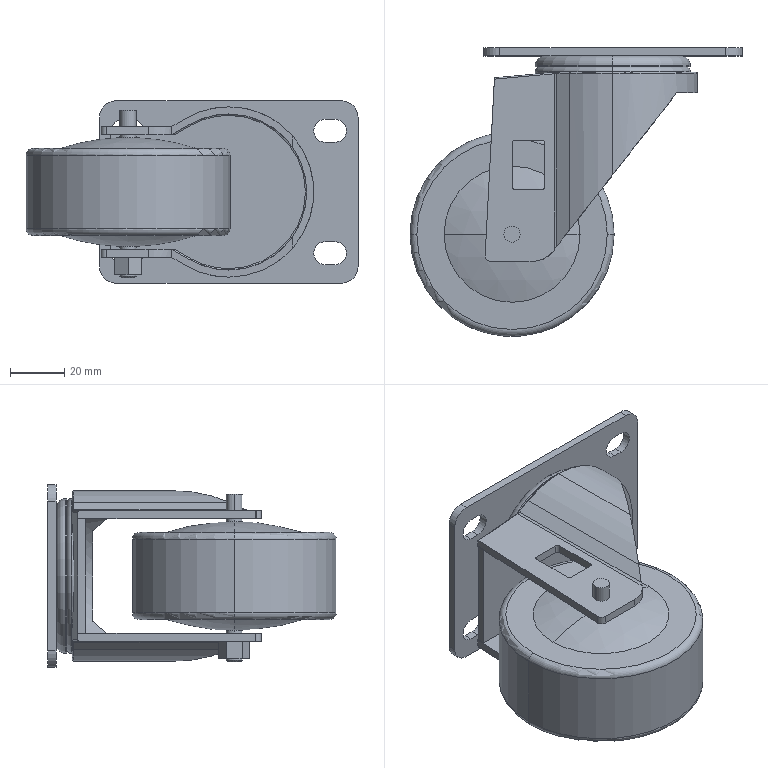Part | STEP file | JDC-75-1 | 1 solid | 137 faces | box 122 x 106 x 67 mm | volume 215545 mm3 | cylinder 56 | plane 55 | torus 16 | spline 4 | sphere 4 | cone 2 | commonest cylinder face diameters 6 x8 8.5 x8 1 x6 4 x5 2 x4 12 x4